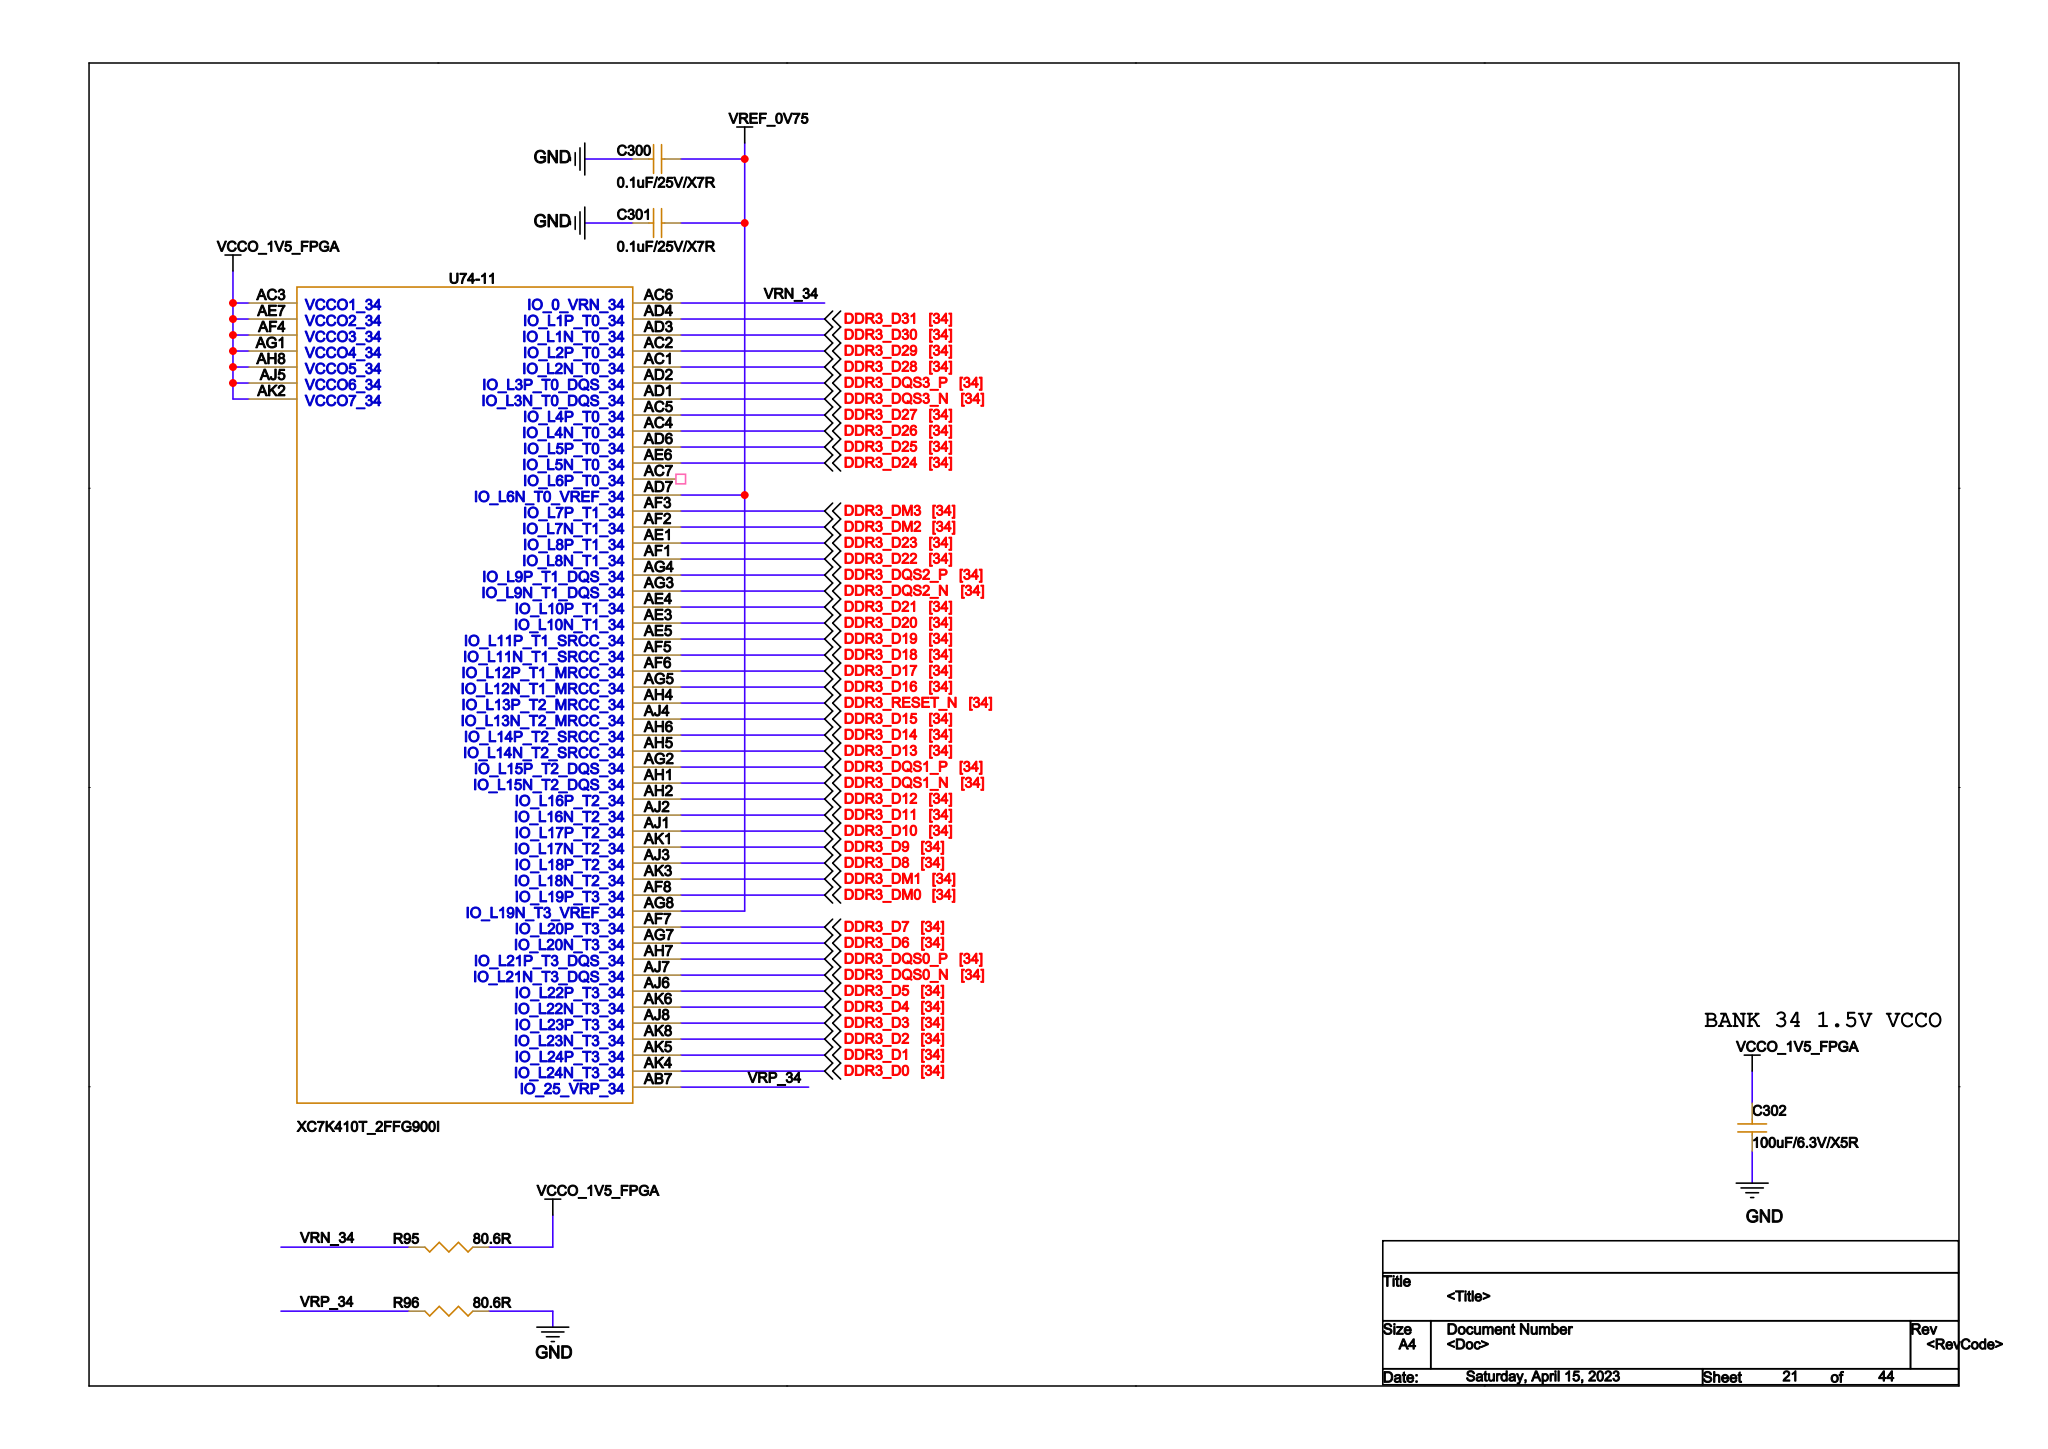Circuit board | Cadence Allegro | 1034 parts | 912 nets | one sheet of the schematic
Parts on this sheet (reference | value | footprint):
C300 | 0.1uF/25V/X7R | C0402_BGA
C301 | 0.1uF/25V/X7R | C0402_BGA
C302 | 100uF/6.3V/X5R | C0402_BGA
R95 | 80.6R | R0402
R96 | 80.6R | R0402
Nets of these parts (net: part-pin ...):
GND: C300-2 C301-2 C302-1 R96-1
VCCO_1V5_FPGA: C302-2 R95-1
VREF_0V75: C300-1 C301-1
VRN_34: R95-2
VRP_34: R96-2